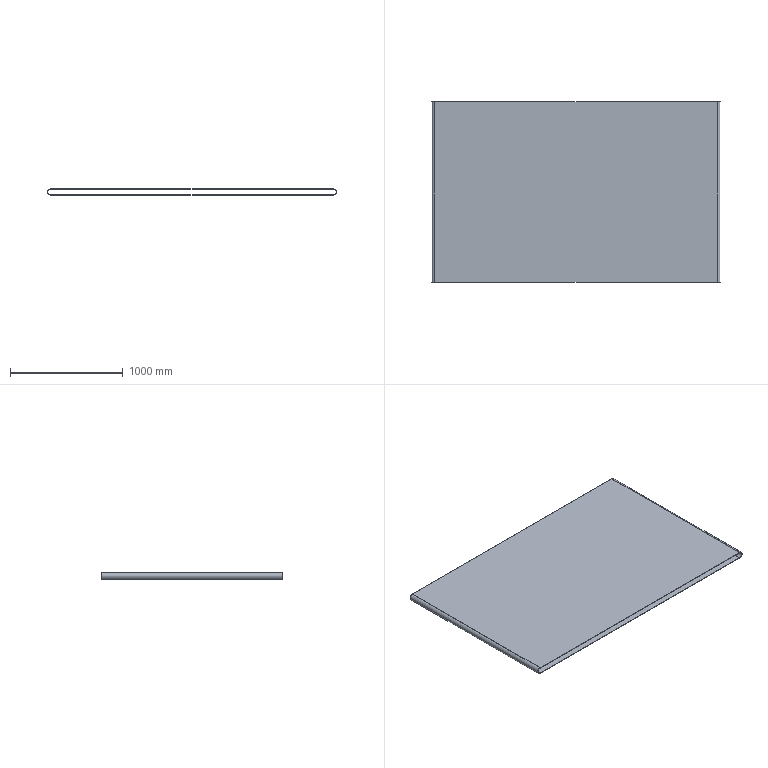Part | STEP file | Belt | 1 solid | 10 faces | box 2560 x 1600 x 60 mm | volume 33125947 mm3 | plane 6 | cylinder 4 | commonest cylinder face diameters 52 x2 60 x2
STEP:
#1=CARTESIAN_POINT('',(0.,1600.,-30.));
#2=VERTEX_POINT('',#1);
#3=CARTESIAN_POINT('',(0.,1600.,30.));
#4=VERTEX_POINT('',#3);
#5=CARTESIAN_POINT('',(0.,1600.,0.));
#6=DIRECTION('',(0.,1.,0.));
#7=DIRECTION('',(0.,0.,1.));
#8=AXIS2_PLACEMENT_3D('',#5,#6,#7);
#9=CIRCLE('',#8,30.);
#10=EDGE_CURVE('',#2,#4,#9,.T.);
#11=ORIENTED_EDGE('',*,*,#10,.T.);
#12=CARTESIAN_POINT('',(2500.,1600.,30.));
#13=VERTEX_POINT('',#12);
#14=CARTESIAN_POINT('',(0.,1600.,30.));
#15=DIRECTION('',(1.,0.,0.));
#16=VECTOR('',#15,1000.);
#17=LINE('',#14,#16);
#18=EDGE_CURVE('',#4,#13,#17,.T.);
#19=ORIENTED_EDGE('',*,*,#18,.T.);
#20=CARTESIAN_POINT('',(2500.,1600.,-30.));
#21=VERTEX_POINT('',#20);
#22=CARTESIAN_POINT('',(2500.,1600.,0.));
#23=DIRECTION('',(0.,1.,0.));
#24=DIRECTION('',(0.,0.,1.));
#25=AXIS2_PLACEMENT_3D('',#22,#23,#24);
#26=CIRCLE('',#25,30.);
#27=EDGE_CURVE('',#13,#21,#26,.T.);
#28=ORIENTED_EDGE('',*,*,#27,.T.);
#29=CARTESIAN_POINT('',(0.,1600.,-30.));
#30=DIRECTION('',(-1.,0.,0.));
#31=VECTOR('',#30,1000.);
#32=LINE('',#29,#31);
#33=EDGE_CURVE('',#21,#2,#32,.T.);
#34=ORIENTED_EDGE('',*,*,#33,.T.);
#35=EDGE_LOOP('',(#11,#19,#28,#34));
#36=FACE_OUTER_BOUND('',#35,.T.);
#37=CARTESIAN_POINT('',(0.,1600.,26.));
#38=VERTEX_POINT('',#37);
#39=CARTESIAN_POINT('',(2500.,1600.,26.));
#40=VERTEX_POINT('',#39);
#41=CARTESIAN_POINT('',(0.,1600.,26.));
#42=DIRECTION('',(1.,0.,0.));
#43=VECTOR('',#42,1000.);
#44=LINE('',#41,#43);
#45=EDGE_CURVE('',#38,#40,#44,.T.);
#46=ORIENTED_EDGE('',*,*,#45,.F.);
#47=CARTESIAN_POINT('',(0.,1600.,-26.));
#48=VERTEX_POINT('',#47);
#49=CARTESIAN_POINT('',(0.,1600.,0.));
#50=DIRECTION('',(0.,1.,0.));
#51=DIRECTION('',(0.,0.,1.));
#52=AXIS2_PLACEMENT_3D('',#49,#50,#51);
#53=CIRCLE('',#52,26.);
#54=EDGE_CURVE('',#48,#38,#53,.T.);
#55=ORIENTED_EDGE('',*,*,#54,.F.);
#56=CARTESIAN_POINT('',(2500.,1600.,-26.));
#57=VERTEX_POINT('',#56);
#58=CARTESIAN_POINT('',(0.,1600.,-26.));
#59=DIRECTION('',(-1.,0.,0.));
#60=VECTOR('',#59,1000.);
#61=LINE('',#58,#60);
#62=EDGE_CURVE('',#57,#48,#61,.T.);
#63=ORIENTED_EDGE('',*,*,#62,.F.);
#64=CARTESIAN_POINT('',(2500.,1600.,0.));
#65=DIRECTION('',(0.,1.,0.));
#66=DIRECTION('',(0.,0.,1.));
#67=AXIS2_PLACEMENT_3D('',#64,#65,#66);
#68=CIRCLE('',#67,26.);
#69=EDGE_CURVE('',#40,#57,#68,.T.);
#70=ORIENTED_EDGE('',*,*,#69,.F.);
#71=EDGE_LOOP('',(#46,#55,#63,#70));
#72=FACE_BOUND('',#71,.T.);
#73=CARTESIAN_POINT('',(0.,1600.,0.));
#74=DIRECTION('',(0.,1.,0.));
#75=DIRECTION('',(0.,0.,1.));
#76=AXIS2_PLACEMENT_3D('',#73,#74,#75);
#77=PLANE('',#76);
#78=ADVANCED_FACE('',(#36,#72),#77,.T.);
#79=CARTESIAN_POINT('',(0.,0.,-30.));
#80=VERTEX_POINT('',#79);
#81=CARTESIAN_POINT('',(0.,0.,30.));
#82=VERTEX_POINT('',#81);
#83=CARTESIAN_POINT('',(0.,0.,0.));
#84=DIRECTION('',(0.,1.,0.));
#85=DIRECTION('',(0.,0.,1.));
#86=AXIS2_PLACEMENT_3D('',#83,#84,#85);
#87=CIRCLE('',#86,30.);
#88=EDGE_CURVE('',#80,#82,#87,.T.);
#89=ORIENTED_EDGE('',*,*,#88,.F.);
#90=CARTESIAN_POINT('',(2500.,0.,-30.));
#91=VERTEX_POINT('',#90);
#92=CARTESIAN_POINT('',(0.,0.,-30.));
#93=DIRECTION('',(-1.,0.,0.));
#94=VECTOR('',#93,1000.);
#95=LINE('',#92,#94);
#96=EDGE_CURVE('',#91,#80,#95,.T.);
#97=ORIENTED_EDGE('',*,*,#96,.F.);
#98=CARTESIAN_POINT('',(2500.,0.,30.));
#99=VERTEX_POINT('',#98);
#100=CARTESIAN_POINT('',(2500.,0.,0.));
#101=DIRECTION('',(0.,1.,0.));
#102=DIRECTION('',(0.,0.,1.));
#103=AXIS2_PLACEMENT_3D('',#100,#101,#102);
#104=CIRCLE('',#103,30.);
#105=EDGE_CURVE('',#99,#91,#104,.T.);
#106=ORIENTED_EDGE('',*,*,#105,.F.);
#107=CARTESIAN_POINT('',(0.,0.,30.));
#108=DIRECTION('',(1.,0.,0.));
#109=VECTOR('',#108,1000.);
#110=LINE('',#107,#109);
#111=EDGE_CURVE('',#82,#99,#110,.T.);
#112=ORIENTED_EDGE('',*,*,#111,.F.);
#113=EDGE_LOOP('',(#89,#97,#106,#112));
#114=FACE_OUTER_BOUND('',#113,.T.);
#115=CARTESIAN_POINT('',(0.,0.,-26.));
#116=VERTEX_POINT('',#115);
#117=CARTESIAN_POINT('',(0.,0.,26.));
#118=VERTEX_POINT('',#117);
#119=CARTESIAN_POINT('',(0.,0.,0.));
#120=DIRECTION('',(0.,1.,0.));
#121=DIRECTION('',(0.,0.,1.));
#122=AXIS2_PLACEMENT_3D('',#119,#120,#121);
#123=CIRCLE('',#122,26.);
#124=EDGE_CURVE('',#116,#118,#123,.T.);
#125=ORIENTED_EDGE('',*,*,#124,.T.);
#126=CARTESIAN_POINT('',(2500.,0.,26.));
#127=VERTEX_POINT('',#126);
#128=CARTESIAN_POINT('',(0.,0.,26.));
#129=DIRECTION('',(1.,0.,0.));
#130=VECTOR('',#129,1000.);
#131=LINE('',#128,#130);
#132=EDGE_CURVE('',#118,#127,#131,.T.);
#133=ORIENTED_EDGE('',*,*,#132,.T.);
#134=CARTESIAN_POINT('',(2500.,0.,-26.));
#135=VERTEX_POINT('',#134);
#136=CARTESIAN_POINT('',(2500.,0.,0.));
#137=DIRECTION('',(0.,1.,0.));
#138=DIRECTION('',(0.,0.,1.));
#139=AXIS2_PLACEMENT_3D('',#136,#137,#138);
#140=CIRCLE('',#139,26.);
#141=EDGE_CURVE('',#127,#135,#140,.T.);
#142=ORIENTED_EDGE('',*,*,#141,.T.);
#143=CARTESIAN_POINT('',(0.,0.,-26.));
#144=DIRECTION('',(-1.,0.,0.));
#145=VECTOR('',#144,1000.);
#146=LINE('',#143,#145);
#147=EDGE_CURVE('',#135,#116,#146,.T.);
#148=ORIENTED_EDGE('',*,*,#147,.T.);
#149=EDGE_LOOP('',(#125,#133,#142,#148));
#150=FACE_BOUND('',#149,.T.);
#151=CARTESIAN_POINT('',(0.,0.,0.));
#152=DIRECTION('',(0.,1.,0.));
#153=DIRECTION('',(0.,0.,1.));
#154=AXIS2_PLACEMENT_3D('',#151,#152,#153);
#155=PLANE('',#154);
#156=ADVANCED_FACE('',(#114,#150),#155,.F.);
#157=ORIENTED_EDGE('',*,*,#88,.T.);
#158=CARTESIAN_POINT('',(0.,1600.,30.));
#159=DIRECTION('',(0.,-1.,0.));
#160=VECTOR('',#159,1000.);
#161=LINE('',#158,#160);
#162=EDGE_CURVE('',#4,#82,#161,.T.);
#163=ORIENTED_EDGE('',*,*,#162,.F.);
#164=ORIENTED_EDGE('',*,*,#10,.F.);
#165=CARTESIAN_POINT('',(0.,1600.,-30.));
#166=DIRECTION('',(0.,-1.,0.));
#167=VECTOR('',#166,1000.);
#168=LINE('',#165,#167);
#169=EDGE_CURVE('',#2,#80,#168,.T.);
#170=ORIENTED_EDGE('',*,*,#169,.T.);
#171=EDGE_LOOP('',(#157,#163,#164,#170));
#172=FACE_OUTER_BOUND('',#171,.T.);
#173=CARTESIAN_POINT('',(0.,1600.,0.));
#174=DIRECTION('',(0.,-1.,0.));
#175=DIRECTION('',(0.,0.,-1.));
#176=AXIS2_PLACEMENT_3D('',#173,#174,#175);
#177=CYLINDRICAL_SURFACE('',#176,30.);
#178=ADVANCED_FACE('',(#172),#177,.T.);
#179=ORIENTED_EDGE('',*,*,#111,.T.);
#180=CARTESIAN_POINT('',(2500.,1600.,30.));
#181=DIRECTION('',(0.,-1.,0.));
#182=VECTOR('',#181,1000.);
#183=LINE('',#180,#182);
#184=EDGE_CURVE('',#13,#99,#183,.T.);
#185=ORIENTED_EDGE('',*,*,#184,.F.);
#186=ORIENTED_EDGE('',*,*,#18,.F.);
#187=ORIENTED_EDGE('',*,*,#162,.T.);
#188=EDGE_LOOP('',(#179,#185,#186,#187));
#189=FACE_OUTER_BOUND('',#188,.T.);
#190=CARTESIAN_POINT('',(0.,1600.,30.));
#191=DIRECTION('',(0.,0.,-1.));
#192=DIRECTION('',(-1.,0.,0.));
#193=AXIS2_PLACEMENT_3D('',#190,#191,#192);
#194=PLANE('',#193);
#195=ADVANCED_FACE('',(#189),#194,.F.);
#196=ORIENTED_EDGE('',*,*,#105,.T.);
#197=CARTESIAN_POINT('',(2500.,1600.,-30.));
#198=DIRECTION('',(0.,-1.,0.));
#199=VECTOR('',#198,1000.);
#200=LINE('',#197,#199);
#201=EDGE_CURVE('',#21,#91,#200,.T.);
#202=ORIENTED_EDGE('',*,*,#201,.F.);
#203=ORIENTED_EDGE('',*,*,#27,.F.);
#204=ORIENTED_EDGE('',*,*,#184,.T.);
#205=EDGE_LOOP('',(#196,#202,#203,#204));
#206=FACE_OUTER_BOUND('',#205,.T.);
#207=CARTESIAN_POINT('',(2500.,1600.,0.));
#208=DIRECTION('',(0.,-1.,0.));
#209=DIRECTION('',(0.,0.,-1.));
#210=AXIS2_PLACEMENT_3D('',#207,#208,#209);
#211=CYLINDRICAL_SURFACE('',#210,30.);
#212=ADVANCED_FACE('',(#206),#211,.T.);
#213=ORIENTED_EDGE('',*,*,#96,.T.);
#214=ORIENTED_EDGE('',*,*,#169,.F.);
#215=ORIENTED_EDGE('',*,*,#33,.F.);
#216=ORIENTED_EDGE('',*,*,#201,.T.);
#217=EDGE_LOOP('',(#213,#214,#215,#216));
#218=FACE_OUTER_BOUND('',#217,.T.);
#219=CARTESIAN_POINT('',(0.,1600.,-30.));
#220=DIRECTION('',(0.,0.,1.));
#221=DIRECTION('',(1.,0.,0.));
#222=AXIS2_PLACEMENT_3D('',#219,#220,#221);
#223=PLANE('',#222);
#224=ADVANCED_FACE('',(#218),#223,.F.);
#225=ORIENTED_EDGE('',*,*,#124,.F.);
#226=CARTESIAN_POINT('',(0.,1600.,-26.));
#227=DIRECTION('',(0.,-1.,0.));
#228=VECTOR('',#227,1000.);
#229=LINE('',#226,#228);
#230=EDGE_CURVE('',#48,#116,#229,.T.);
#231=ORIENTED_EDGE('',*,*,#230,.F.);
#232=ORIENTED_EDGE('',*,*,#54,.T.);
#233=CARTESIAN_POINT('',(0.,1600.,26.));
#234=DIRECTION('',(0.,-1.,0.));
#235=VECTOR('',#234,1000.);
#236=LINE('',#233,#235);
#237=EDGE_CURVE('',#38,#118,#236,.T.);
#238=ORIENTED_EDGE('',*,*,#237,.T.);
#239=EDGE_LOOP('',(#225,#231,#232,#238));
#240=FACE_OUTER_BOUND('',#239,.T.);
#241=CARTESIAN_POINT('',(0.,1600.,0.));
#242=DIRECTION('',(0.,-1.,0.));
#243=DIRECTION('',(0.,0.,-1.));
#244=AXIS2_PLACEMENT_3D('',#241,#242,#243);
#245=CYLINDRICAL_SURFACE('',#244,26.);
#246=ADVANCED_FACE('',(#240),#245,.F.);
#247=ORIENTED_EDGE('',*,*,#132,.F.);
#248=ORIENTED_EDGE('',*,*,#237,.F.);
#249=ORIENTED_EDGE('',*,*,#45,.T.);
#250=CARTESIAN_POINT('',(2500.,1600.,26.));
#251=DIRECTION('',(0.,-1.,0.));
#252=VECTOR('',#251,1000.);
#253=LINE('',#250,#252);
#254=EDGE_CURVE('',#40,#127,#253,.T.);
#255=ORIENTED_EDGE('',*,*,#254,.T.);
#256=EDGE_LOOP('',(#247,#248,#249,#255));
#257=FACE_OUTER_BOUND('',#256,.T.);
#258=CARTESIAN_POINT('',(0.,1600.,26.));
#259=DIRECTION('',(0.,0.,-1.));
#260=DIRECTION('',(-1.,0.,0.));
#261=AXIS2_PLACEMENT_3D('',#258,#259,#260);
#262=PLANE('',#261);
#263=ADVANCED_FACE('',(#257),#262,.T.);
#264=ORIENTED_EDGE('',*,*,#141,.F.);
#265=ORIENTED_EDGE('',*,*,#254,.F.);
#266=ORIENTED_EDGE('',*,*,#69,.T.);
#267=CARTESIAN_POINT('',(2500.,1600.,-26.));
#268=DIRECTION('',(0.,-1.,0.));
#269=VECTOR('',#268,1000.);
#270=LINE('',#267,#269);
#271=EDGE_CURVE('',#57,#135,#270,.T.);
#272=ORIENTED_EDGE('',*,*,#271,.T.);
#273=EDGE_LOOP('',(#264,#265,#266,#272));
#274=FACE_OUTER_BOUND('',#273,.T.);
#275=CARTESIAN_POINT('',(2500.,1600.,0.));
#276=DIRECTION('',(0.,-1.,0.));
#277=DIRECTION('',(0.,0.,-1.));
#278=AXIS2_PLACEMENT_3D('',#275,#276,#277);
#279=CYLINDRICAL_SURFACE('',#278,26.);
#280=ADVANCED_FACE('',(#274),#279,.F.);
#281=ORIENTED_EDGE('',*,*,#147,.F.);
#282=ORIENTED_EDGE('',*,*,#271,.F.);
#283=ORIENTED_EDGE('',*,*,#62,.T.);
#284=ORIENTED_EDGE('',*,*,#230,.T.);
#285=EDGE_LOOP('',(#281,#282,#283,#284));
#286=FACE_OUTER_BOUND('',#285,.T.);
#287=CARTESIAN_POINT('',(0.,1600.,-26.));
#288=DIRECTION('',(0.,0.,1.));
#289=DIRECTION('',(1.,0.,0.));
#290=AXIS2_PLACEMENT_3D('',#287,#288,#289);
#291=PLANE('',#290);
#292=ADVANCED_FACE('',(#286),#291,.T.);
#293=CLOSED_SHELL('',(#78,#156,#178,#195,#212,#224,#246,#263,#280,#292));
#294=MANIFOLD_SOLID_BREP('',#293);
#295=CARTESIAN_POINT('',(0.,0.,0.));
#296=DIRECTION('',(0.,0.,1.));
#297=DIRECTION('',(1.,0.,0.));
#298=AXIS2_PLACEMENT_3D('',#295,#296,#297);
#299=(LENGTH_UNIT()NAMED_UNIT(*)SI_UNIT(.MILLI.,.METRE.));
#300=UNCERTAINTY_MEASURE_WITH_UNIT(LENGTH_MEASURE(0.00001),#299,'','');
#301=(NAMED_UNIT(*)PLANE_ANGLE_UNIT()SI_UNIT($,.RADIAN.));
#302=(NAMED_UNIT(*)SI_UNIT($,.STERADIAN.)SOLID_ANGLE_UNIT());
#303=(GEOMETRIC_REPRESENTATION_CONTEXT(3)GLOBAL_UNCERTAINTY_ASSIGNED_CONTEXT((#300))GLOBAL_UNIT_ASSIGNED_CONTEXT((#299,#301,#302))REPRESENTATION_CONTEXT('',''));
#304=ADVANCED_BREP_SHAPE_REPRESENTATION('',(#294,#298),#303);